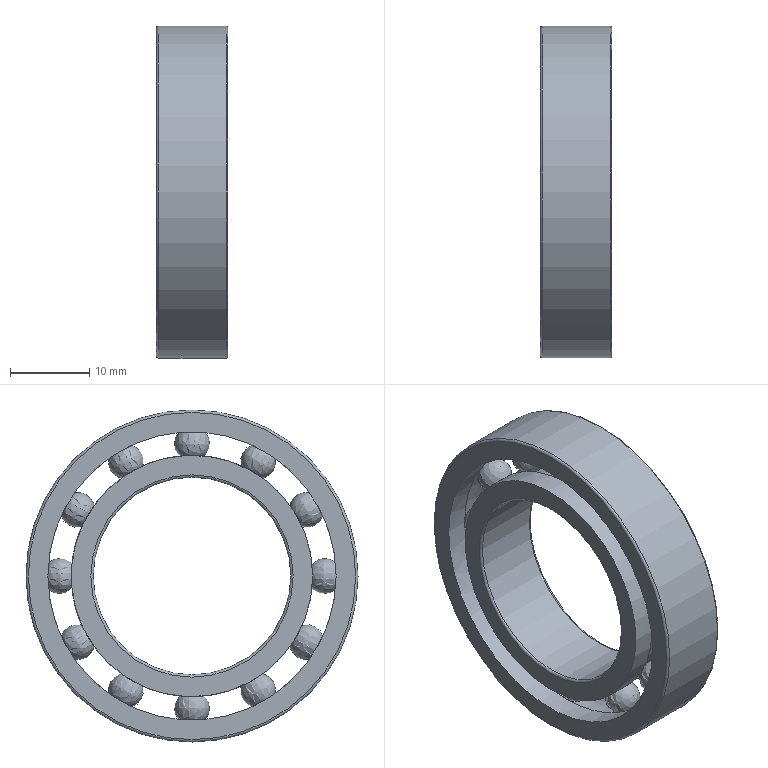Part | STEP file | Rolling bearing 70000AC 71905 AC GB_T 292 | 14 solids | 50 faces | box 9 x 42 x 42 mm | volume 5353 mm3 | torus 28 | sphere 12 | cylinder 5 | plane 4 | cone 1 | commonest cylinder face diameters 30.542 x2 25 x1 36.458 x1 42 x1